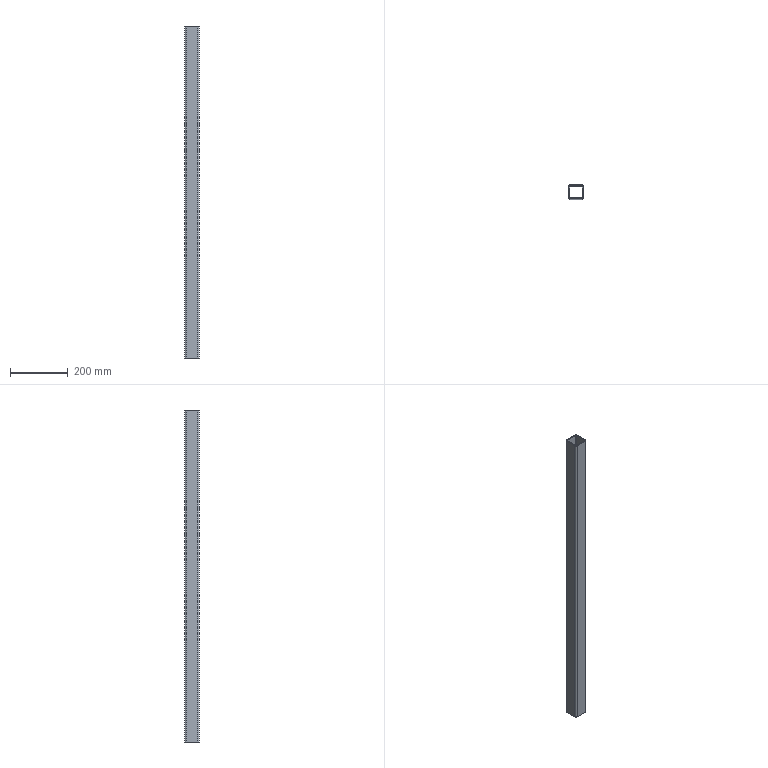Part | STEP file | Square steel 50×50×1150 | 1 solid | 18 faces | box 50 x 50 x 1150 mm | volume 822708 mm3 | plane 10 | cylinder 8 | commonest cylinder face diameters 2 x4 10 x4
STEP:
#1=CARTESIAN_POINT('',(0.,0.,0.));
#2=DIRECTION('',(0.,0.,1.));
#3=DIRECTION('',(1.,0.,0.));
#4=AXIS2_PLACEMENT_3D('',#1,#2,#3);
#5=CARTESIAN_POINT('',(-25.,-20.,575.));
#6=VERTEX_POINT('',#5);
#7=CARTESIAN_POINT('',(-20.,-25.,575.));
#8=VERTEX_POINT('',#7);
#9=CARTESIAN_POINT('',(-20.,-20.,575.));
#10=DIRECTION('',(0.,0.,1.));
#11=DIRECTION('',(1.,0.,0.));
#12=AXIS2_PLACEMENT_3D('',#9,#10,#11);
#13=CIRCLE('',#12,5.);
#14=CARTESIAN_POINT('',(-20.,-20.,575.));
#15=DIRECTION('',(0.,0.,1.));
#16=DIRECTION('',(1.,0.,0.));
#17=AXIS2_PLACEMENT_3D('',#14,#15,#16);
#18=PLANE('',#17);
#19=CARTESIAN_POINT('',(0.,0.));
#20=DIRECTION('',(1.,0.));
#21=AXIS2_PLACEMENT_2D('',#19,#20);
#22=CIRCLE('',#21,5.);
#23=(GEOMETRIC_REPRESENTATION_CONTEXT(2)PARAMETRIC_REPRESENTATION_CONTEXT()REPRESENTATION_CONTEXT('',''));
#24=DEFINITIONAL_REPRESENTATION('',(#22),#23);
#25=PCURVE('',#18,#24);
#26=CARTESIAN_POINT('',(-20.,-20.,575.));
#27=DIRECTION('',(0.,0.,-1.));
#28=DIRECTION('',(-1.,0.,0.));
#29=AXIS2_PLACEMENT_3D('',#26,#27,#28);
#30=CYLINDRICAL_SURFACE('',#29,5.);
#31=CARTESIAN_POINT('',(9.425,0.));
#32=DIRECTION('',(-1.,0.));
#33=VECTOR('',#32,1.);
#34=LINE('',#31,#33);
#35=(GEOMETRIC_REPRESENTATION_CONTEXT(2)PARAMETRIC_REPRESENTATION_CONTEXT()REPRESENTATION_CONTEXT('',''));
#36=DEFINITIONAL_REPRESENTATION('',(#34),#35);
#37=PCURVE('',#30,#36);
#38=SURFACE_CURVE('',#13,(#25,#37),.PCURVE_S1.);
#39=EDGE_CURVE('',#6,#8,#38,.T.);
#40=ORIENTED_EDGE('',*,*,#39,.T.);
#41=CARTESIAN_POINT('',(20.,-25.,575.));
#42=VERTEX_POINT('',#41);
#43=CARTESIAN_POINT('',(-20.,-25.,575.));
#44=DIRECTION('',(1.,0.,0.));
#45=VECTOR('',#44,1.);
#46=LINE('',#43,#45);
#47=CARTESIAN_POINT('',(0.,-5.));
#48=DIRECTION('',(1.,0.));
#49=VECTOR('',#48,1.);
#50=LINE('',#47,#49);
#51=(GEOMETRIC_REPRESENTATION_CONTEXT(2)PARAMETRIC_REPRESENTATION_CONTEXT()REPRESENTATION_CONTEXT('',''));
#52=DEFINITIONAL_REPRESENTATION('',(#50),#51);
#53=PCURVE('',#18,#52);
#54=CARTESIAN_POINT('',(-20.,-25.,575.));
#55=DIRECTION('',(0.,1.,0.));
#56=DIRECTION('',(0.,0.,1.));
#57=AXIS2_PLACEMENT_3D('',#54,#55,#56);
#58=PLANE('',#57);
#59=CARTESIAN_POINT('',(0.,0.));
#60=DIRECTION('',(0.,1.));
#61=VECTOR('',#60,1.);
#62=LINE('',#59,#61);
#63=(GEOMETRIC_REPRESENTATION_CONTEXT(2)PARAMETRIC_REPRESENTATION_CONTEXT()REPRESENTATION_CONTEXT('',''));
#64=DEFINITIONAL_REPRESENTATION('',(#62),#63);
#65=PCURVE('',#58,#64);
#66=SURFACE_CURVE('',#46,(#53,#65),.PCURVE_S1.);
#67=EDGE_CURVE('',#8,#42,#66,.T.);
#68=ORIENTED_EDGE('',*,*,#67,.T.);
#69=CARTESIAN_POINT('',(25.,-20.,575.));
#70=VERTEX_POINT('',#69);
#71=CARTESIAN_POINT('',(20.,-20.,575.));
#72=DIRECTION('',(0.,0.,1.));
#73=DIRECTION('',(-1.,0.,0.));
#74=AXIS2_PLACEMENT_3D('',#71,#72,#73);
#75=CIRCLE('',#74,5.);
#76=CARTESIAN_POINT('',(40.,0.));
#77=DIRECTION('',(-1.,0.));
#78=AXIS2_PLACEMENT_2D('',#76,#77);
#79=CIRCLE('',#78,5.);
#80=(GEOMETRIC_REPRESENTATION_CONTEXT(2)PARAMETRIC_REPRESENTATION_CONTEXT()REPRESENTATION_CONTEXT('',''));
#81=DEFINITIONAL_REPRESENTATION('',(#79),#80);
#82=PCURVE('',#18,#81);
#83=CARTESIAN_POINT('',(20.,-20.,575.));
#84=DIRECTION('',(0.,0.,-1.));
#85=DIRECTION('',(-1.,0.,0.));
#86=AXIS2_PLACEMENT_3D('',#83,#84,#85);
#87=CYLINDRICAL_SURFACE('',#86,5.);
#88=CARTESIAN_POINT('',(6.283,0.));
#89=DIRECTION('',(-1.,0.));
#90=VECTOR('',#89,1.);
#91=LINE('',#88,#90);
#92=(GEOMETRIC_REPRESENTATION_CONTEXT(2)PARAMETRIC_REPRESENTATION_CONTEXT()REPRESENTATION_CONTEXT('',''));
#93=DEFINITIONAL_REPRESENTATION('',(#91),#92);
#94=PCURVE('',#87,#93);
#95=SURFACE_CURVE('',#75,(#82,#94),.PCURVE_S1.);
#96=EDGE_CURVE('',#42,#70,#95,.T.);
#97=ORIENTED_EDGE('',*,*,#96,.T.);
#98=CARTESIAN_POINT('',(25.,20.,575.));
#99=VERTEX_POINT('',#98);
#100=CARTESIAN_POINT('',(25.,20.,575.));
#101=DIRECTION('',(0.,1.,0.));
#102=VECTOR('',#101,1.);
#103=LINE('',#100,#102);
#104=CARTESIAN_POINT('',(45.,40.));
#105=DIRECTION('',(0.,1.));
#106=VECTOR('',#105,1.);
#107=LINE('',#104,#106);
#108=(GEOMETRIC_REPRESENTATION_CONTEXT(2)PARAMETRIC_REPRESENTATION_CONTEXT()REPRESENTATION_CONTEXT('',''));
#109=DEFINITIONAL_REPRESENTATION('',(#107),#108);
#110=PCURVE('',#18,#109);
#111=CARTESIAN_POINT('',(25.,20.,575.));
#112=DIRECTION('',(-1.,0.,0.));
#113=DIRECTION('',(0.,-1.,0.));
#114=AXIS2_PLACEMENT_3D('',#111,#112,#113);
#115=PLANE('',#114);
#116=CARTESIAN_POINT('',(0.,0.));
#117=DIRECTION('',(-1.,0.));
#118=VECTOR('',#117,1.);
#119=LINE('',#116,#118);
#120=(GEOMETRIC_REPRESENTATION_CONTEXT(2)PARAMETRIC_REPRESENTATION_CONTEXT()REPRESENTATION_CONTEXT('',''));
#121=DEFINITIONAL_REPRESENTATION('',(#119),#120);
#122=PCURVE('',#115,#121);
#123=SURFACE_CURVE('',#103,(#110,#122),.PCURVE_S1.);
#124=EDGE_CURVE('',#70,#99,#123,.T.);
#125=ORIENTED_EDGE('',*,*,#124,.T.);
#126=CARTESIAN_POINT('',(20.,25.,575.));
#127=VERTEX_POINT('',#126);
#128=CARTESIAN_POINT('',(20.,20.,575.));
#129=DIRECTION('',(0.,0.,1.));
#130=DIRECTION('',(1.,0.,0.));
#131=AXIS2_PLACEMENT_3D('',#128,#129,#130);
#132=CIRCLE('',#131,5.);
#133=CARTESIAN_POINT('',(40.,40.));
#134=DIRECTION('',(1.,0.));
#135=AXIS2_PLACEMENT_2D('',#133,#134);
#136=CIRCLE('',#135,5.);
#137=(GEOMETRIC_REPRESENTATION_CONTEXT(2)PARAMETRIC_REPRESENTATION_CONTEXT()REPRESENTATION_CONTEXT('',''));
#138=DEFINITIONAL_REPRESENTATION('',(#136),#137);
#139=PCURVE('',#18,#138);
#140=CARTESIAN_POINT('',(20.,20.,575.));
#141=DIRECTION('',(0.,0.,-1.));
#142=DIRECTION('',(-1.,0.,0.));
#143=AXIS2_PLACEMENT_3D('',#140,#141,#142);
#144=CYLINDRICAL_SURFACE('',#143,5.);
#145=CARTESIAN_POINT('',(3.142,0.));
#146=DIRECTION('',(-1.,0.));
#147=VECTOR('',#146,1.);
#148=LINE('',#145,#147);
#149=(GEOMETRIC_REPRESENTATION_CONTEXT(2)PARAMETRIC_REPRESENTATION_CONTEXT()REPRESENTATION_CONTEXT('',''));
#150=DEFINITIONAL_REPRESENTATION('',(#148),#149);
#151=PCURVE('',#144,#150);
#152=SURFACE_CURVE('',#132,(#139,#151),.PCURVE_S1.);
#153=EDGE_CURVE('',#99,#127,#152,.T.);
#154=ORIENTED_EDGE('',*,*,#153,.T.);
#155=CARTESIAN_POINT('',(-20.,25.,575.));
#156=VERTEX_POINT('',#155);
#157=CARTESIAN_POINT('',(-20.,25.,575.));
#158=DIRECTION('',(-1.,0.,0.));
#159=VECTOR('',#158,1.);
#160=LINE('',#157,#159);
#161=CARTESIAN_POINT('',(0.,45.));
#162=DIRECTION('',(-1.,0.));
#163=VECTOR('',#162,1.);
#164=LINE('',#161,#163);
#165=(GEOMETRIC_REPRESENTATION_CONTEXT(2)PARAMETRIC_REPRESENTATION_CONTEXT()REPRESENTATION_CONTEXT('',''));
#166=DEFINITIONAL_REPRESENTATION('',(#164),#165);
#167=PCURVE('',#18,#166);
#168=CARTESIAN_POINT('',(-20.,25.,575.));
#169=DIRECTION('',(0.,-1.,0.));
#170=DIRECTION('',(0.,0.,-1.));
#171=AXIS2_PLACEMENT_3D('',#168,#169,#170);
#172=PLANE('',#171);
#173=CARTESIAN_POINT('',(0.,0.));
#174=DIRECTION('',(0.,-1.));
#175=VECTOR('',#174,1.);
#176=LINE('',#173,#175);
#177=(GEOMETRIC_REPRESENTATION_CONTEXT(2)PARAMETRIC_REPRESENTATION_CONTEXT()REPRESENTATION_CONTEXT('',''));
#178=DEFINITIONAL_REPRESENTATION('',(#176),#177);
#179=PCURVE('',#172,#178);
#180=SURFACE_CURVE('',#160,(#167,#179),.PCURVE_S1.);
#181=EDGE_CURVE('',#127,#156,#180,.T.);
#182=ORIENTED_EDGE('',*,*,#181,.T.);
#183=CARTESIAN_POINT('',(-25.,20.,575.));
#184=VERTEX_POINT('',#183);
#185=CARTESIAN_POINT('',(-20.,20.,575.));
#186=DIRECTION('',(0.,0.,1.));
#187=DIRECTION('',(-1.,0.,0.));
#188=AXIS2_PLACEMENT_3D('',#185,#186,#187);
#189=CIRCLE('',#188,5.);
#190=CARTESIAN_POINT('',(0.,40.));
#191=DIRECTION('',(-1.,0.));
#192=AXIS2_PLACEMENT_2D('',#190,#191);
#193=CIRCLE('',#192,5.);
#194=(GEOMETRIC_REPRESENTATION_CONTEXT(2)PARAMETRIC_REPRESENTATION_CONTEXT()REPRESENTATION_CONTEXT('',''));
#195=DEFINITIONAL_REPRESENTATION('',(#193),#194);
#196=PCURVE('',#18,#195);
#197=CARTESIAN_POINT('',(-20.,20.,575.));
#198=DIRECTION('',(0.,0.,-1.));
#199=DIRECTION('',(-1.,0.,0.));
#200=AXIS2_PLACEMENT_3D('',#197,#198,#199);
#201=CYLINDRICAL_SURFACE('',#200,5.);
#202=CARTESIAN_POINT('',(6.283,0.));
#203=DIRECTION('',(-1.,0.));
#204=VECTOR('',#203,1.);
#205=LINE('',#202,#204);
#206=(GEOMETRIC_REPRESENTATION_CONTEXT(2)PARAMETRIC_REPRESENTATION_CONTEXT()REPRESENTATION_CONTEXT('',''));
#207=DEFINITIONAL_REPRESENTATION('',(#205),#206);
#208=PCURVE('',#201,#207);
#209=SURFACE_CURVE('',#189,(#196,#208),.PCURVE_S1.);
#210=EDGE_CURVE('',#156,#184,#209,.T.);
#211=ORIENTED_EDGE('',*,*,#210,.T.);
#212=CARTESIAN_POINT('',(-25.,20.,575.));
#213=DIRECTION('',(0.,-1.,0.));
#214=VECTOR('',#213,1.);
#215=LINE('',#212,#214);
#216=CARTESIAN_POINT('',(-5.,40.));
#217=DIRECTION('',(0.,-1.));
#218=VECTOR('',#217,1.);
#219=LINE('',#216,#218);
#220=(GEOMETRIC_REPRESENTATION_CONTEXT(2)PARAMETRIC_REPRESENTATION_CONTEXT()REPRESENTATION_CONTEXT('',''));
#221=DEFINITIONAL_REPRESENTATION('',(#219),#220);
#222=PCURVE('',#18,#221);
#223=CARTESIAN_POINT('',(-25.,20.,575.));
#224=DIRECTION('',(1.,0.,0.));
#225=DIRECTION('',(0.,1.,0.));
#226=AXIS2_PLACEMENT_3D('',#223,#224,#225);
#227=PLANE('',#226);
#228=CARTESIAN_POINT('',(0.,0.));
#229=DIRECTION('',(-1.,0.));
#230=VECTOR('',#229,1.);
#231=LINE('',#228,#230);
#232=(GEOMETRIC_REPRESENTATION_CONTEXT(2)PARAMETRIC_REPRESENTATION_CONTEXT()REPRESENTATION_CONTEXT('',''));
#233=DEFINITIONAL_REPRESENTATION('',(#231),#232);
#234=PCURVE('',#227,#233);
#235=SURFACE_CURVE('',#215,(#222,#234),.PCURVE_S1.);
#236=EDGE_CURVE('',#184,#6,#235,.T.);
#237=ORIENTED_EDGE('',*,*,#236,.T.);
#238=EDGE_LOOP('',(#40,#68,#97,#125,#154,#182,#211,#237));
#239=FACE_BOUND('',#238,.T.);
#240=CARTESIAN_POINT('',(-21.,20.,575.));
#241=VERTEX_POINT('',#240);
#242=CARTESIAN_POINT('',(-21.,-20.,575.));
#243=VERTEX_POINT('',#242);
#244=CARTESIAN_POINT('',(-21.,20.,575.));
#245=DIRECTION('',(0.,-1.,0.));
#246=VECTOR('',#245,1.);
#247=LINE('',#244,#246);
#248=CARTESIAN_POINT('',(-1.,40.));
#249=DIRECTION('',(0.,-1.));
#250=VECTOR('',#249,1.);
#251=LINE('',#248,#250);
#252=(GEOMETRIC_REPRESENTATION_CONTEXT(2)PARAMETRIC_REPRESENTATION_CONTEXT()REPRESENTATION_CONTEXT('',''));
#253=DEFINITIONAL_REPRESENTATION('',(#251),#252);
#254=PCURVE('',#18,#253);
#255=CARTESIAN_POINT('',(-21.,20.,575.));
#256=DIRECTION('',(1.,0.,0.));
#257=DIRECTION('',(0.,1.,0.));
#258=AXIS2_PLACEMENT_3D('',#255,#256,#257);
#259=PLANE('',#258);
#260=CARTESIAN_POINT('',(0.,0.));
#261=DIRECTION('',(-1.,0.));
#262=VECTOR('',#261,1.);
#263=LINE('',#260,#262);
#264=(GEOMETRIC_REPRESENTATION_CONTEXT(2)PARAMETRIC_REPRESENTATION_CONTEXT()REPRESENTATION_CONTEXT('',''));
#265=DEFINITIONAL_REPRESENTATION('',(#263),#264);
#266=PCURVE('',#259,#265);
#267=SURFACE_CURVE('',#247,(#254,#266),.PCURVE_S1.);
#268=EDGE_CURVE('',#241,#243,#267,.T.);
#269=ORIENTED_EDGE('',*,*,#268,.F.);
#270=CARTESIAN_POINT('',(-20.,21.,575.));
#271=VERTEX_POINT('',#270);
#272=CARTESIAN_POINT('',(-20.,20.,575.));
#273=DIRECTION('',(0.,0.,1.));
#274=DIRECTION('',(-1.,0.,0.));
#275=AXIS2_PLACEMENT_3D('',#272,#273,#274);
#276=CIRCLE('',#275,1.);
#277=CARTESIAN_POINT('',(0.,40.));
#278=DIRECTION('',(-1.,0.));
#279=AXIS2_PLACEMENT_2D('',#277,#278);
#280=CIRCLE('',#279,1.);
#281=(GEOMETRIC_REPRESENTATION_CONTEXT(2)PARAMETRIC_REPRESENTATION_CONTEXT()REPRESENTATION_CONTEXT('',''));
#282=DEFINITIONAL_REPRESENTATION('',(#280),#281);
#283=PCURVE('',#18,#282);
#284=CARTESIAN_POINT('',(-20.,20.,575.));
#285=DIRECTION('',(0.,0.,-1.));
#286=DIRECTION('',(-1.,0.,0.));
#287=AXIS2_PLACEMENT_3D('',#284,#285,#286);
#288=CYLINDRICAL_SURFACE('',#287,1.);
#289=CARTESIAN_POINT('',(6.283,0.));
#290=DIRECTION('',(-1.,0.));
#291=VECTOR('',#290,1.);
#292=LINE('',#289,#291);
#293=(GEOMETRIC_REPRESENTATION_CONTEXT(2)PARAMETRIC_REPRESENTATION_CONTEXT()REPRESENTATION_CONTEXT('',''));
#294=DEFINITIONAL_REPRESENTATION('',(#292),#293);
#295=PCURVE('',#288,#294);
#296=SURFACE_CURVE('',#276,(#283,#295),.PCURVE_S1.);
#297=EDGE_CURVE('',#271,#241,#296,.T.);
#298=ORIENTED_EDGE('',*,*,#297,.F.);
#299=CARTESIAN_POINT('',(20.,21.,575.));
#300=VERTEX_POINT('',#299);
#301=CARTESIAN_POINT('',(-20.,21.,575.));
#302=DIRECTION('',(-1.,0.,0.));
#303=VECTOR('',#302,1.);
#304=LINE('',#301,#303);
#305=CARTESIAN_POINT('',(0.,41.));
#306=DIRECTION('',(-1.,0.));
#307=VECTOR('',#306,1.);
#308=LINE('',#305,#307);
#309=(GEOMETRIC_REPRESENTATION_CONTEXT(2)PARAMETRIC_REPRESENTATION_CONTEXT()REPRESENTATION_CONTEXT('',''));
#310=DEFINITIONAL_REPRESENTATION('',(#308),#309);
#311=PCURVE('',#18,#310);
#312=CARTESIAN_POINT('',(-20.,21.,575.));
#313=DIRECTION('',(0.,-1.,0.));
#314=DIRECTION('',(0.,0.,-1.));
#315=AXIS2_PLACEMENT_3D('',#312,#313,#314);
#316=PLANE('',#315);
#317=CARTESIAN_POINT('',(0.,0.));
#318=DIRECTION('',(0.,-1.));
#319=VECTOR('',#318,1.);
#320=LINE('',#317,#319);
#321=(GEOMETRIC_REPRESENTATION_CONTEXT(2)PARAMETRIC_REPRESENTATION_CONTEXT()REPRESENTATION_CONTEXT('',''));
#322=DEFINITIONAL_REPRESENTATION('',(#320),#321);
#323=PCURVE('',#316,#322);
#324=SURFACE_CURVE('',#304,(#311,#323),.PCURVE_S1.);
#325=EDGE_CURVE('',#300,#271,#324,.T.);
#326=ORIENTED_EDGE('',*,*,#325,.F.);
#327=CARTESIAN_POINT('',(21.,20.,575.));
#328=VERTEX_POINT('',#327);
#329=CARTESIAN_POINT('',(20.,20.,575.));
#330=DIRECTION('',(0.,0.,1.));
#331=DIRECTION('',(1.,0.,0.));
#332=AXIS2_PLACEMENT_3D('',#329,#330,#331);
#333=CIRCLE('',#332,1.);
#334=CARTESIAN_POINT('',(40.,40.));
#335=DIRECTION('',(1.,0.));
#336=AXIS2_PLACEMENT_2D('',#334,#335);
#337=CIRCLE('',#336,1.);
#338=(GEOMETRIC_REPRESENTATION_CONTEXT(2)PARAMETRIC_REPRESENTATION_CONTEXT()REPRESENTATION_CONTEXT('',''));
#339=DEFINITIONAL_REPRESENTATION('',(#337),#338);
#340=PCURVE('',#18,#339);
#341=CARTESIAN_POINT('',(20.,20.,575.));
#342=DIRECTION('',(0.,0.,-1.));
#343=DIRECTION('',(-1.,0.,0.));
#344=AXIS2_PLACEMENT_3D('',#341,#342,#343);
#345=CYLINDRICAL_SURFACE('',#344,1.);
#346=CARTESIAN_POINT('',(3.142,0.));
#347=DIRECTION('',(-1.,0.));
#348=VECTOR('',#347,1.);
#349=LINE('',#346,#348);
#350=(GEOMETRIC_REPRESENTATION_CONTEXT(2)PARAMETRIC_REPRESENTATION_CONTEXT()REPRESENTATION_CONTEXT('',''));
#351=DEFINITIONAL_REPRESENTATION('',(#349),#350);
#352=PCURVE('',#345,#351);
#353=SURFACE_CURVE('',#333,(#340,#352),.PCURVE_S1.);
#354=EDGE_CURVE('',#328,#300,#353,.T.);
#355=ORIENTED_EDGE('',*,*,#354,.F.);
#356=CARTESIAN_POINT('',(21.,-20.,575.));
#357=VERTEX_POINT('',#356);
#358=CARTESIAN_POINT('',(21.,20.,575.));
#359=DIRECTION('',(0.,1.,0.));
#360=VECTOR('',#359,1.);
#361=LINE('',#358,#360);
#362=CARTESIAN_POINT('',(41.,40.));
#363=DIRECTION('',(0.,1.));
#364=VECTOR('',#363,1.);
#365=LINE('',#362,#364);
#366=(GEOMETRIC_REPRESENTATION_CONTEXT(2)PARAMETRIC_REPRESENTATION_CONTEXT()REPRESENTATION_CONTEXT('',''));
#367=DEFINITIONAL_REPRESENTATION('',(#365),#366);
#368=PCURVE('',#18,#367);
#369=CARTESIAN_POINT('',(21.,20.,575.));
#370=DIRECTION('',(-1.,0.,0.));
#371=DIRECTION('',(0.,0.,1.));
#372=AXIS2_PLACEMENT_3D('',#369,#370,#371);
#373=PLANE('',#372);
#374=CARTESIAN_POINT('',(0.,0.));
#375=DIRECTION('',(0.,1.));
#376=VECTOR('',#375,1.);
#377=LINE('',#374,#376);
#378=(GEOMETRIC_REPRESENTATION_CONTEXT(2)PARAMETRIC_REPRESENTATION_CONTEXT()REPRESENTATION_CONTEXT('',''));
#379=DEFINITIONAL_REPRESENTATION('',(#377),#378);
#380=PCURVE('',#373,#379);
#381=SURFACE_CURVE('',#361,(#368,#380),.PCURVE_S1.);
#382=EDGE_CURVE('',#357,#328,#381,.T.);
#383=ORIENTED_EDGE('',*,*,#382,.F.);
#384=CARTESIAN_POINT('',(20.,-21.,575.));
#385=VERTEX_POINT('',#384);
#386=CARTESIAN_POINT('',(20.,-20.,575.));
#387=DIRECTION('',(0.,0.,1.));
#388=DIRECTION('',(-1.,0.,0.));
#389=AXIS2_PLACEMENT_3D('',#386,#387,#388);
#390=CIRCLE('',#389,1.);
#391=CARTESIAN_POINT('',(40.,0.));
#392=DIRECTION('',(-1.,0.));
#393=AXIS2_PLACEMENT_2D('',#391,#392);
#394=CIRCLE('',#393,1.);
#395=(GEOMETRIC_REPRESENTATION_CONTEXT(2)PARAMETRIC_REPRESENTATION_CONTEXT()REPRESENTATION_CONTEXT('',''));
#396=DEFINITIONAL_REPRESENTATION('',(#394),#395);
#397=PCURVE('',#18,#396);
#398=CARTESIAN_POINT('',(20.,-20.,575.));
#399=DIRECTION('',(0.,0.,-1.));
#400=DIRECTION('',(-1.,0.,0.));
#401=AXIS2_PLACEMENT_3D('',#398,#399,#400);
#402=CYLINDRICAL_SURFACE('',#401,1.);
#403=CARTESIAN_POINT('',(6.283,0.));
#404=DIRECTION('',(-1.,0.));
#405=VECTOR('',#404,1.);
#406=LINE('',#403,#405);
#407=(GEOMETRIC_REPRESENTATION_CONTEXT(2)PARAMETRIC_REPRESENTATION_CONTEXT()REPRESENTATION_CONTEXT('',''));
#408=DEFINITIONAL_REPRESENTATION('',(#406),#407);
#409=PCURVE('',#402,#408);
#410=SURFACE_CURVE('',#390,(#397,#409),.PCURVE_S1.);
#411=EDGE_CURVE('',#385,#357,#410,.T.);
#412=ORIENTED_EDGE('',*,*,#411,.F.);
#413=CARTESIAN_POINT('',(-20.,-21.,575.));
#414=VERTEX_POINT('',#413);
#415=CARTESIAN_POINT('',(-20.,-21.,575.));
#416=DIRECTION('',(1.,0.,0.));
#417=VECTOR('',#416,1.);
#418=LINE('',#415,#417);
#419=CARTESIAN_POINT('',(0.,-1.));
#420=DIRECTION('',(1.,0.));
#421=VECTOR('',#420,1.);
#422=LINE('',#419,#421);
#423=(GEOMETRIC_REPRESENTATION_CONTEXT(2)PARAMETRIC_REPRESENTATION_CONTEXT()REPRESENTATION_CONTEXT('',''));
#424=DEFINITIONAL_REPRESENTATION('',(#422),#423);
#425=PCURVE('',#18,#424);
#426=CARTESIAN_POINT('',(-20.,-21.,575.));
#427=DIRECTION('',(0.,1.,0.));
#428=DIRECTION('',(0.,0.,1.));
#429=AXIS2_PLACEMENT_3D('',#426,#427,#428);
#430=PLANE('',#429);
#431=CARTESIAN_POINT('',(0.,0.));
#432=DIRECTION('',(0.,1.));
#433=VECTOR('',#432,1.);
#434=LINE('',#431,#433);
#435=(GEOMETRIC_REPRESENTATION_CONTEXT(2)PARAMETRIC_REPRESENTATION_CONTEXT()REPRESENTATION_CONTEXT('',''));
#436=DEFINITIONAL_REPRESENTATION('',(#434),#435);
#437=PCURVE('',#430,#436);
#438=SURFACE_CURVE('',#418,(#425,#437),.PCURVE_S1.);
#439=EDGE_CURVE('',#414,#385,#438,.T.);
#440=ORIENTED_EDGE('',*,*,#439,.F.);
#441=CARTESIAN_POINT('',(-20.,-20.,575.));
#442=DIRECTION('',(0.,0.,1.));
#443=DIRECTION('',(1.,0.,0.));
#444=AXIS2_PLACEMENT_3D('',#441,#442,#443);
#445=CIRCLE('',#444,1.);
#446=CARTESIAN_POINT('',(0.,0.));
#447=DIRECTION('',(1.,0.));
#448=AXIS2_PLACEMENT_2D('',#446,#447);
#449=CIRCLE('',#448,1.);
#450=(GEOMETRIC_REPRESENTATION_CONTEXT(2)PARAMETRIC_REPRESENTATION_CONTEXT()REPRESENTATION_CONTEXT('',''));
#451=DEFINITIONAL_REPRESENTATION('',(#449),#450);
#452=PCURVE('',#18,#451);
#453=CARTESIAN_POINT('',(-20.,-20.,575.));
#454=DIRECTION('',(0.,0.,-1.));
#455=DIRECTION('',(-1.,0.,0.));
#456=AXIS2_PLACEMENT_3D('',#453,#454,#455);
#457=CYLINDRICAL_SURFACE('',#456,1.);
#458=CARTESIAN_POINT('',(9.425,0.));
#459=DIRECTION('',(-1.,0.));
#460=VECTOR('',#459,1.);
#461=LINE('',#458,#460);
#462=(GEOMETRIC_REPRESENTATION_CONTEXT(2)PARAMETRIC_REPRESENTATION_CONTEXT()REPRESENTATION_CONTEXT('',''));
#463=DEFINITIONAL_REPRESENTATION('',(#461),#462);
#464=PCURVE('',#457,#463);
#465=SURFACE_CURVE('',#445,(#452,#464),.PCURVE_S1.);
#466=EDGE_CURVE('',#243,#414,#465,.T.);
#467=ORIENTED_EDGE('',*,*,#466,.F.);
#468=EDGE_LOOP('',(#269,#298,#326,#355,#383,#412,#440,#467));
#469=FACE_BOUND('',#468,.T.);
#470=ADVANCED_FACE('',(#239,#469),#18,.T.);
#471=CARTESIAN_POINT('',(-25.,-20.,-575.));
#472=VERTEX_POINT('',#471);
#473=CARTESIAN_POINT('',(-20.,-25.,-575.));
#474=VERTEX_POINT('',#473);
#475=CARTESIAN_POINT('',(-20.,-20.,-575.));
#476=DIRECTION('',(0.,0.,1.));
#477=DIRECTION('',(1.,0.,0.));
#478=AXIS2_PLACEMENT_3D('',#475,#476,#477);
#479=CIRCLE('',#478,5.);
#480=CARTESIAN_POINT('',(-20.,-20.,-575.));
#481=DIRECTION('',(0.,0.,1.));
#482=DIRECTION('',(1.,0.,0.));
#483=AXIS2_PLACEMENT_3D('',#480,#481,#482);
#484=PLANE('',#483);
#485=CARTESIAN_POINT('',(0.,0.));
#486=DIRECTION('',(1.,0.));
#487=AXIS2_PLACEMENT_2D('',#485,#486);
#488=CIRCLE('',#487,5.);
#489=(GEOMETRIC_REPRESENTATION_CONTEXT(2)PARAMETRIC_REPRESENTATION_CONTEXT()REPRESENTATION_CONTEXT('',''));
#490=DEFINITIONAL_REPRESENTATION('',(#488),#489);
#491=PCURVE('',#484,#490);
#492=CARTESIAN_POINT('',(9.425,1150.));
#493=DIRECTION('',(-1.,0.));
#494=VECTOR('',#493,1.);
#495=LINE('',#492,#494);
#496=(GEOMETRIC_REPRESENTATION_CONTEXT(2)PARAMETRIC_REPRESENTATION_CONTEXT()REPRESENTATION_CONTEXT('',''));
#497=DEFINITIONAL_REPRESENTATION('',(#495),#496);
#498=PCURVE('',#30,#497);
#499=SURFACE_CURVE('',#479,(#491,#498),.PCURVE_S1.);
#500=EDGE_CURVE('',#472,#474,#499,.T.);
#501=ORIENTED_EDGE('',*,*,#500,.F.);
#502=CARTESIAN_POINT('',(-25.,20.,-575.));
#503=VERTEX_POINT('',#502);
#504=CARTESIAN_POINT('',(-25.,20.,-575.));
#505=DIRECTION('',(0.,-1.,0.));
#506=VECTOR('',#505,1.);
#507=LINE('',#504,#506);
#508=CARTESIAN_POINT('',(-5.,40.));
#509=DIRECTION('',(0.,-1.));
#510=VECTOR('',#509,1.);
#511=LINE('',#508,#510);
#512=(GEOMETRIC_REPRESENTATION_CONTEXT(2)PARAMETRIC_REPRESENTATION_CONTEXT()REPRESENTATION_CONTEXT('',''));
#513=DEFINITIONAL_REPRESENTATION('',(#511),#512);
#514=PCURVE('',#484,#513);
#515=CARTESIAN_POINT('',(0.,-1150.));
#516=DIRECTION('',(-1.,0.));
#517=VECTOR('',#516,1.);
#518=LINE('',#515,#517);
#519=(GEOMETRIC_REPRESENTATION_CONTEXT(2)PARAMETRIC_REPRESENTATION_CONTEXT()REPRESENTATION_CONTEXT('',''));
#520=DEFINITIONAL_REPRESENTATION('',(#518),#519);
#521=PCURVE('',#227,#520);
#522=SURFACE_CURVE('',#507,(#514,#521),.PCURVE_S1.);
#523=EDGE_CURVE('',#503,#472,#522,.T.);
#524=ORIENTED_EDGE('',*,*,#523,.F.);
#525=CARTESIAN_POINT('',(-20.,25.,-575.));
#526=VERTEX_POINT('',#525);
#527=CARTESIAN_POINT('',(-20.,20.,-575.));
#528=DIRECTION('',(0.,0.,1.));
#529=DIRECTION('',(-1.,0.,0.));
#530=AXIS2_PLACEMENT_3D('',#527,#528,#529);
#531=CIRCLE('',#530,5.);
#532=CARTESIAN_POINT('',(0.,40.));
#533=DIRECTION('',(-1.,0.));
#534=AXIS2_PLACEMENT_2D('',#532,#533);
#535=CIRCLE('',#534,5.);
#536=(GEOMETRIC_REPRESENTATION_CONTEXT(2)PARAMETRIC_REPRESENTATION_CONTEXT()REPRESENTATION_CONTEXT('',''));
#537=DEFINITIONAL_REPRESENTATION('',(#535),#536);
#538=PCURVE('',#484,#537);
#539=CARTESIAN_POINT('',(6.283,1150.));
#540=DIRECTION('',(-1.,0.));
#541=VECTOR('',#540,1.);
#542=LINE('',#539,#541);
#543=(GEOMETRIC_REPRESENTATION_CONTEXT(2)PARAMETRIC_REPRESENTATION_CONTEXT()REPRESENTATION_CONTEXT('',''));
#544=DEFINITIONAL_REPRESENTATION('',(#542),#543);
#545=PCURVE('',#201,#544);
#546=SURFACE_CURVE('',#531,(#538,#545),.PCURVE_S1.);
#547=EDGE_CURVE('',#526,#503,#546,.T.);
#548=ORIENTED_EDGE('',*,*,#547,.F.);
#549=CARTESIAN_POINT('',(20.,25.,-575.));
#550=VERTEX_POINT('',#549);
#551=CARTESIAN_POINT('',(-20.,25.,-575.));
#552=DIRECTION('',(-1.,0.,0.));
#553=VECTOR('',#552,1.);
#554=LINE('',#551,#553);
#555=CARTESIAN_POINT('',(0.,45.));
#556=DIRECTION('',(-1.,0.));
#557=VECTOR('',#556,1.);
#558=LINE('',#555,#557);
#559=(GEOMETRIC_REPRESENTATION_CONTEXT(2)PARAMETRIC_REPRESENTATION_CONTEXT()REPRESENTATION_CONTEXT('',''));
#560=DEFINITIONAL_REPRESENTATION('',(#558),#559);
#561=PCURVE('',#484,#560);
#562=CARTESIAN_POINT('',(1150.,0.));
#563=DIRECTION('',(0.,-1.));
#564=VECTOR('',#563,1.);
#565=LINE('',#562,#564);
#566=(GEOMETRIC_REPRESENTATION_CONTEXT(2)PARAMETRIC_REPRESENTATION_CONTEXT()REPRESENTATION_CONTEXT('',''));
#567=DEFINITIONAL_REPRESENTATION('',(#565),#566);
#568=PCURVE('',#172,#567);
#569=SURFACE_CURVE('',#554,(#561,#568),.PCURVE_S1.);
#570=EDGE_CURVE('',#550,#526,#569,.T.);
#571=ORIENTED_EDGE('',*,*,#570,.F.);
#572=CARTESIAN_POINT('',(25.,20.,-575.));
#573=VERTEX_POINT('',#572);
#574=CARTESIAN_POINT('',(20.,20.,-575.));
#575=DIRECTION('',(0.,0.,1.));
#576=DIRECTION('',(1.,0.,0.));
#577=AXIS2_PLACEMENT_3D('',#574,#575,#576);
#578=CIRCLE('',#577,5.);
#579=CARTESIAN_POINT('',(40.,40.));
#580=DIRECTION('',(1.,0.));
#581=AXIS2_PLACEMENT_2D('',#579,#580);
#582=CIRCLE('',#581,5.);
#583=(GEOMETRIC_REPRESENTATION_CONTEXT(2)PARAMETRIC_REPRESENTATION_CONTEXT()REPRESENTATION_CONTEXT('',''));
#584=DEFINITIONAL_REPRESENTATION('',(#582),#583);
#585=PCURVE('',#484,#584);
#586=CARTESIAN_POINT('',(3.142,1150.));
#587=DIRECTION('',(-1.,0.));
#588=VECTOR('',#587,1.);
#589=LINE('',#586,#588);
#590=(GEOMETRIC_REPRESENTATION_CONTEXT(2)PARAMETRIC_REPRESENTATION_CONTEXT()REPRESENTATION_CONTEXT('',''));
#591=DEFINITIONAL_REPRESENTATION('',(#589),#590);
#592=PCURVE('',#144,#591);
#593=SURFACE_CURVE('',#578,(#585,#592),.PCURVE_S1.);
#594=EDGE_CURVE('',#573,#550,#593,.T.);
#595=ORIENTED_EDGE('',*,*,#594,.F.);
#596=CARTESIAN_POINT('',(25.,-20.,-575.));
#597=VERTEX_POINT('',#596);
#598=CARTESIAN_POINT('',(25.,20.,-575.));
#599=DIRECTION('',(0.,1.,0.));
#600=VECTOR('',#599,1.);
#601=LINE('',#598,#600);
#602=CARTESIAN_POINT('',(45.,40.));
#603=DIRECTION('',(0.,1.));
#604=VECTOR('',#603,1.);
#605=LINE('',#602,#604);
#606=(GEOMETRIC_REPRESENTATION_CONTEXT(2)PARAMETRIC_REPRESENTATION_CONTEXT()REPRESENTATION_CONTEXT('',''));
#607=DEFINITIONAL_REPRESENTATION('',(#605),#606);
#608=PCURVE('',#484,#607);
#609=CARTESIAN_POINT('',(0.,-1150.));
#610=DIRECTION('',(-1.,0.));
#611=VECTOR('',#610,1.);
#612=LINE('',#609,#611);
#613=(GEOMETRIC_REPRESENTATION_CONTEXT(2)PARAMETRIC_REPRESENTATION_CONTEXT()REPRESENTATION_CONTEXT('',''));
#614=DEFINITIONAL_REPRESENTATION('',(#612),#613);
#615=PCURVE('',#115,#614);
#616=SURFACE_CURVE('',#601,(#608,#615),.PCURVE_S1.);
#617=EDGE_CURVE('',#597,#573,#616,.T.);
#618=ORIENTED_EDGE('',*,*,#617,.F.);
#619=CARTESIAN_POINT('',(20.,-25.,-575.));
#620=VERTEX_POINT('',#619);
#621=CARTESIAN_POINT('',(20.,-20.,-575.));
#622=DIRECTION('',(0.,0.,1.));
#623=DIRECTION('',(-1.,0.,0.));
#624=AXIS2_PLACEMENT_3D('',#621,#622,#623);
#625=CIRCLE('',#624,5.);
#626=CARTESIAN_POINT('',(40.,0.));
#627=DIRECTION('',(-1.,0.));
#628=AXIS2_PLACEMENT_2D('',#626,#627);
#629=CIRCLE('',#628,5.);
#630=(GEOMETRIC_REPRESENTATION_CONTEXT(2)PARAMETRIC_REPRESENTATION_CONTEXT()REPRESENTATION_CONTEXT('',''));
#631=DEFINITIONAL_REPRESENTATION('',(#629),#630);
#632=PCURVE('',#484,#631);
#633=CARTESIAN_POINT('',(6.283,1150.));
#634=DIRECTION('',(-1.,0.));
#635=VECTOR('',#634,1.);
#636=LINE('',#633,#635);
#637=(GEOMETRIC_REPRESENTATION_CONTEXT(2)PARAMETRIC_REPRESENTATION_CONTEXT()REPRESENTATION_CONTEXT('',''));
#638=DEFINITIONAL_REPRESENTATION('',(#636),#637);
#639=PCURVE('',#87,#638);
#640=SURFACE_CURVE('',#625,(#632,#639),.PCURVE_S1.);
#641=EDGE_CURVE('',#620,#597,#640,.T.);
#642=ORIENTED_EDGE('',*,*,#641,.F.);
#643=CARTESIAN_POINT('',(-20.,-25.,-575.));
#644=DIRECTION('',(1.,0.,0.));
#645=VECTOR('',#644,1.);
#646=LINE('',#643,#645);
#647=CARTESIAN_POINT('',(0.,-5.));
#648=DIRECTION('',(1.,0.));
#649=VECTOR('',#648,1.);
#650=LINE('',#647,#649);
#651=(GEOMETRIC_REPRESENTATION_CONTEXT(2)PARAMETRIC_REPRESENTATION_CONTEXT()REPRESENTATION_CONTEXT('',''));
#652=DEFINITIONAL_REPRESENTATION('',(#650),#651);
#653=PCURVE('',#484,#652);
#654=CARTESIAN_POINT('',(-1150.,0.));
#655=DIRECTION('',(0.,1.));
#656=VECTOR('',#655,1.);
#657=LINE('',#654,#656);
#658=(GEOMETRIC_REPRESENTATION_CONTEXT(2)PARAMETRIC_REPRESENTATION_CONTEXT()REPRESENTATION_CONTEXT('',''));
#659=DEFINITIONAL_REPRESENTATION('',(#657),#658);
#660=PCURVE('',#58,#659);
#661=SURFACE_CURVE('',#646,(#653,#660),.PCURVE_S1.);
#662=EDGE_CURVE('',#474,#620,#661,.T.);
#663=ORIENTED_EDGE('',*,*,#662,.F.);
#664=EDGE_LOOP('',(#501,#524,#548,#571,#595,#618,#642,#663));
#665=FACE_BOUND('',#664,.T.);
#666=CARTESIAN_POINT('',(-20.,21.,-575.));
#667=VERTEX_POINT('',#666);
#668=CARTESIAN_POINT('',(-21.,20.,-575.));
#669=VERTEX_POINT('',#668);
#670=CARTESIAN_POINT('',(-20.,20.,-575.));
#671=DIRECTION('',(0.,0.,1.));
#672=DIRECTION('',(-1.,0.,0.));
#673=AXIS2_PLACEMENT_3D('',#670,#671,#672);
#674=CIRCLE('',#673,1.);
#675=CARTESIAN_POINT('',(0.,40.));
#676=DIRECTION('',(-1.,0.));
#677=AXIS2_PLACEMENT_2D('',#675,#676);
#678=CIRCLE('',#677,1.);
#679=(GEOMETRIC_REPRESENTATION_CONTEXT(2)PARAMETRIC_REPRESENTATION_CONTEXT()REPRESENTATION_CONTEXT('',''));
#680=DEFINITIONAL_REPRESENTATION('',(#678),#679);
#681=PCURVE('',#484,#680);
#682=CARTESIAN_POINT('',(6.283,1150.));
#683=DIRECTION('',(-1.,0.));
#684=VECTOR('',#683,1.);
#685=LINE('',#682,#684);
#686=(GEOMETRIC_REPRESENTATION_CONTEXT(2)PARAMETRIC_REPRESENTATION_CONTEXT()REPRESENTATION_CONTEXT('',''));
#687=DEFINITIONAL_REPRESENTATION('',(#685),#686);
#688=PCURVE('',#288,#687);
#689=SURFACE_CURVE('',#674,(#681,#688),.PCURVE_S1.);
#690=EDGE_CURVE('',#667,#669,#689,.T.);
#691=ORIENTED_EDGE('',*,*,#690,.T.);
#692=CARTESIAN_POINT('',(-21.,-20.,-575.));
#693=VERTEX_POINT('',#692);
#694=CARTESIAN_POINT('',(-21.,20.,-575.));
#695=DIRECTION('',(0.,-1.,0.));
#696=VECTOR('',#695,1.);
#697=LINE('',#694,#696);
#698=CARTESIAN_POINT('',(-1.,40.));
#699=DIRECTION('',(0.,-1.));
#700=VECTOR('',#699,1.);
#701=LINE('',#698,#700);
#702=(GEOMETRIC_REPRESENTATION_CONTEXT(2)PARAMETRIC_REPRESENTATION_CONTEXT()REPRESENTATION_CONTEXT('',''));
#703=DEFINITIONAL_REPRESENTATION('',(#701),#702);
#704=PCURVE('',#484,#703);
#705=CARTESIAN_POINT('',(0.,-1150.));
#706=DIRECTION('',(-1.,0.));
#707=VECTOR('',#706,1.);
#708=LINE('',#705,#707);
#709=(GEOMETRIC_REPRESENTATION_CONTEXT(2)PARAMETRIC_REPRESENTATION_CONTEXT()REPRESENTATION_CONTEXT('',''));
#710=DEFINITIONAL_REPRESENTATION('',(#708),#709);
#711=PCURVE('',#259,#710);
#712=SURFACE_CURVE('',#697,(#704,#711),.PCURVE_S1.);
#713=EDGE_CURVE('',#669,#693,#712,.T.);
#714=ORIENTED_EDGE('',*,*,#713,.T.);
#715=CARTESIAN_POINT('',(-20.,-21.,-575.));
#716=VERTEX_POINT('',#715);
#717=CARTESIAN_POINT('',(-20.,-20.,-575.));
#718=DIRECTION('',(0.,0.,1.));
#719=DIRECTION('',(1.,0.,0.));
#720=AXIS2_PLACEMENT_3D('',#717,#718,#719);
#721=CIRCLE('',#720,1.);
#722=CARTESIAN_POINT('',(0.,0.));
#723=DIRECTION('',(1.,0.));
#724=AXIS2_PLACEMENT_2D('',#722,#723);
#725=CIRCLE('',#724,1.);
#726=(GEOMETRIC_REPRESENTATION_CONTEXT(2)PARAMETRIC_REPRESENTATION_CONTEXT()REPRESENTATION_CONTEXT('',''));
#727=DEFINITIONAL_REPRESENTATION('',(#725),#726);
#728=PCURVE('',#484,#727);
#729=CARTESIAN_POINT('',(9.425,1150.));
#730=DIRECTION('',(-1.,0.));
#731=VECTOR('',#730,1.);
#732=LINE('',#729,#731);
#733=(GEOMETRIC_REPRESENTATION_CONTEXT(2)PARAMETRIC_REPRESENTATION_CONTEXT()REPRESENTATION_CONTEXT('',''));
#734=DEFINITIONAL_REPRESENTATION('',(#732),#733);
#735=PCURVE('',#457,#734);
#736=SURFACE_CURVE('',#721,(#728,#735),.PCURVE_S1.);
#737=EDGE_CURVE('',#693,#716,#736,.T.);
#738=ORIENTED_EDGE('',*,*,#737,.T.);
#739=CARTESIAN_POINT('',(20.,-21.,-575.));
#740=VERTEX_POINT('',#739);
#741=CARTESIAN_POINT('',(-20.,-21.,-575.));
#742=DIRECTION('',(1.,0.,0.));
#743=VECTOR('',#742,1.);
#744=LINE('',#741,#743);
#745=CARTESIAN_POINT('',(0.,-1.));
#746=DIRECTION('',(1.,0.));
#747=VECTOR('',#746,1.);
#748=LINE('',#745,#747);
#749=(GEOMETRIC_REPRESENTATION_CONTEXT(2)PARAMETRIC_REPRESENTATION_CONTEXT()REPRESENTATION_CONTEXT('',''));
#750=DEFINITIONAL_REPRESENTATION('',(#748),#749);
#751=PCURVE('',#484,#750);
#752=CARTESIAN_POINT('',(-1150.,0.));
#753=DIRECTION('',(0.,1.));
#754=VECTOR('',#753,1.);
#755=LINE('',#752,#754);
#756=(GEOMETRIC_REPRESENTATION_CONTEXT(2)PARAMETRIC_REPRESENTATION_CONTEXT()REPRESENTATION_CONTEXT('',''));
#757=DEFINITIONAL_REPRESENTATION('',(#755),#756);
#758=PCURVE('',#430,#757);
#759=SURFACE_CURVE('',#744,(#751,#758),.PCURVE_S1.);
#760=EDGE_CURVE('',#716,#740,#759,.T.);
#761=ORIENTED_EDGE('',*,*,#760,.T.);
#762=CARTESIAN_POINT('',(21.,-20.,-575.));
#763=VERTEX_POINT('',#762);
#764=CARTESIAN_POINT('',(20.,-20.,-575.));
#765=DIRECTION('',(0.,0.,1.));
#766=DIRECTION('',(-1.,0.,0.));
#767=AXIS2_PLACEMENT_3D('',#764,#765,#766);
#768=CIRCLE('',#767,1.);
#769=CARTESIAN_POINT('',(40.,0.));
#770=DIRECTION('',(-1.,0.));
#771=AXIS2_PLACEMENT_2D('',#769,#770);
#772=CIRCLE('',#771,1.);
#773=(GEOMETRIC_REPRESENTATION_CONTEXT(2)PARAMETRIC_REPRESENTATION_CONTEXT()REPRESENTATION_CONTEXT('',''));
#774=DEFINITIONAL_REPRESENTATION('',(#772),#773);
#775=PCURVE('',#484,#774);
#776=CARTESIAN_POINT('',(6.283,1150.));
#777=DIRECTION('',(-1.,0.));
#778=VECTOR('',#777,1.);
#779=LINE('',#776,#778);
#780=(GEOMETRIC_REPRESENTATION_CONTEXT(2)PARAMETRIC_REPRESENTATION_CONTEXT()REPRESENTATION_CONTEXT('',''));
#781=DEFINITIONAL_REPRESENTATION('',(#779),#780);
#782=PCURVE('',#402,#781);
#783=SURFACE_CURVE('',#768,(#775,#782),.PCURVE_S1.);
#784=EDGE_CURVE('',#740,#763,#783,.T.);
#785=ORIENTED_EDGE('',*,*,#784,.T.);
#786=CARTESIAN_POINT('',(21.,20.,-575.));
#787=VERTEX_POINT('',#786);
#788=CARTESIAN_POINT('',(21.,20.,-575.));
#789=DIRECTION('',(0.,1.,0.));
#790=VECTOR('',#789,1.);
#791=LINE('',#788,#790);
#792=CARTESIAN_POINT('',(41.,40.));
#793=DIRECTION('',(0.,1.));
#794=VECTOR('',#793,1.);
#795=LINE('',#792,#794);
#796=(GEOMETRIC_REPRESENTATION_CONTEXT(2)PARAMETRIC_REPRESENTATION_CONTEXT()REPRESENTATION_CONTEXT('',''));
#797=DEFINITIONAL_REPRESENTATION('',(#795),#796);
#798=PCURVE('',#484,#797);
#799=CARTESIAN_POINT('',(-1150.,0.));
#800=DIRECTION('',(0.,1.));
#801=VECTOR('',#800,1.);
#802=LINE('',#799,#801);
#803=(GEOMETRIC_REPRESENTATION_CONTEXT(2)PARAMETRIC_REPRESENTATION_CONTEXT()REPRESENTATION_CONTEXT('',''));
#804=DEFINITIONAL_REPRESENTATION('',(#802),#803);
#805=PCURVE('',#373,#804);
#806=SURFACE_CURVE('',#791,(#798,#805),.PCURVE_S1.);
#807=EDGE_CURVE('',#763,#787,#806,.T.);
#808=ORIENTED_EDGE('',*,*,#807,.T.);
#809=CARTESIAN_POINT('',(20.,21.,-575.));
#810=VERTEX_POINT('',#809);
#811=CARTESIAN_POINT('',(20.,20.,-575.));
#812=DIRECTION('',(0.,0.,1.));
#813=DIRECTION('',(1.,0.,0.));
#814=AXIS2_PLACEMENT_3D('',#811,#812,#813);
#815=CIRCLE('',#814,1.);
#816=CARTESIAN_POINT('',(40.,40.));
#817=DIRECTION('',(1.,0.));
#818=AXIS2_PLACEMENT_2D('',#816,#817);
#819=CIRCLE('',#818,1.);
#820=(GEOMETRIC_REPRESENTATION_CONTEXT(2)PARAMETRIC_REPRESENTATION_CONTEXT()REPRESENTATION_CONTEXT('',''));
#821=DEFINITIONAL_REPRESENTATION('',(#819),#820);
#822=PCURVE('',#484,#821);
#823=CARTESIAN_POINT('',(3.142,1150.));
#824=DIRECTION('',(-1.,0.));
#825=VECTOR('',#824,1.);
#826=LINE('',#823,#825);
#827=(GEOMETRIC_REPRESENTATION_CONTEXT(2)PARAMETRIC_REPRESENTATION_CONTEXT()REPRESENTATION_CONTEXT('',''));
#828=DEFINITIONAL_REPRESENTATION('',(#826),#827);
#829=PCURVE('',#345,#828);
#830=SURFACE_CURVE('',#815,(#822,#829),.PCURVE_S1.);
#831=EDGE_CURVE('',#787,#810,#830,.T.);
#832=ORIENTED_EDGE('',*,*,#831,.T.);
#833=CARTESIAN_POINT('',(-20.,21.,-575.));
#834=DIRECTION('',(-1.,0.,0.));
#835=VECTOR('',#834,1.);
#836=LINE('',#833,#835);
#837=CARTESIAN_POINT('',(0.,41.));
#838=DIRECTION('',(-1.,0.));
#839=VECTOR('',#838,1.);
#840=LINE('',#837,#839);
#841=(GEOMETRIC_REPRESENTATION_CONTEXT(2)PARAMETRIC_REPRESENTATION_CONTEXT()REPRESENTATION_CONTEXT('',''));
#842=DEFINITIONAL_REPRESENTATION('',(#840),#841);
#843=PCURVE('',#484,#842);
#844=CARTESIAN_POINT('',(1150.,0.));
#845=DIRECTION('',(0.,-1.));
#846=VECTOR('',#845,1.);
#847=LINE('',#844,#846);
#848=(GEOMETRIC_REPRESENTATION_CONTEXT(2)PARAMETRIC_REPRESENTATION_CONTEXT()REPRESENTATION_CONTEXT('',''));
#849=DEFINITIONAL_REPRESENTATION('',(#847),#848);
#850=PCURVE('',#316,#849);
#851=SURFACE_CURVE('',#836,(#843,#850),.PCURVE_S1.);
#852=EDGE_CURVE('',#810,#667,#851,.T.);
#853=ORIENTED_EDGE('',*,*,#852,.T.);
#854=EDGE_LOOP('',(#691,#714,#738,#761,#785,#808,#832,#853));
#855=FACE_BOUND('',#854,.T.);
#856=ADVANCED_FACE('',(#665,#855),#484,.F.);
#857=ORIENTED_EDGE('',*,*,#500,.T.);
#858=CARTESIAN_POINT('',(-20.,-25.,575.));
#859=DIRECTION('',(0.,0.,-1.));
#860=VECTOR('',#859,1.);
#861=LINE('',#858,#860);
#862=CARTESIAN_POINT('',(4.712,0.));
#863=DIRECTION('',(0.,1.));
#864=VECTOR('',#863,1.);
#865=LINE('',#862,#864);
#866=(GEOMETRIC_REPRESENTATION_CONTEXT(2)PARAMETRIC_REPRESENTATION_CONTEXT()REPRESENTATION_CONTEXT('',''));
#867=DEFINITIONAL_REPRESENTATION('',(#865),#866);
#868=PCURVE('',#30,#867);
#869=CARTESIAN_POINT('',(0.,0.));
#870=DIRECTION('',(-1.,0.));
#871=VECTOR('',#870,1.);
#872=LINE('',#869,#871);
#873=(GEOMETRIC_REPRESENTATION_CONTEXT(2)PARAMETRIC_REPRESENTATION_CONTEXT()REPRESENTATION_CONTEXT('',''));
#874=DEFINITIONAL_REPRESENTATION('',(#872),#873);
#875=PCURVE('',#58,#874);
#876=SURFACE_CURVE('',#861,(#868,#875),.PCURVE_S1.);
#877=EDGE_CURVE('',#8,#474,#876,.T.);
#878=ORIENTED_EDGE('',*,*,#877,.F.);
#879=ORIENTED_EDGE('',*,*,#39,.F.);
#880=CARTESIAN_POINT('',(-25.,-20.,575.));
#881=DIRECTION('',(0.,0.,-1.));
#882=VECTOR('',#881,1.);
#883=LINE('',#880,#882);
#884=CARTESIAN_POINT('',(6.283,0.));
#885=DIRECTION('',(0.,1.));
#886=VECTOR('',#885,1.);
#887=LINE('',#884,#886);
#888=(GEOMETRIC_REPRESENTATION_CONTEXT(2)PARAMETRIC_REPRESENTATION_CONTEXT()REPRESENTATION_CONTEXT('',''));
#889=DEFINITIONAL_REPRESENTATION('',(#887),#888);
#890=PCURVE('',#30,#889);
#891=CARTESIAN_POINT('',(-40.,0.));
#892=DIRECTION('',(0.,-1.));
#893=VECTOR('',#892,1.);
#894=LINE('',#891,#893);
#895=(GEOMETRIC_REPRESENTATION_CONTEXT(2)PARAMETRIC_REPRESENTATION_CONTEXT()REPRESENTATION_CONTEXT('',''));
#896=DEFINITIONAL_REPRESENTATION('',(#894),#895);
#897=PCURVE('',#227,#896);
#898=SURFACE_CURVE('',#883,(#890,#897),.PCURVE_S1.);
#899=EDGE_CURVE('',#6,#472,#898,.T.);
#900=ORIENTED_EDGE('',*,*,#899,.T.);
#901=EDGE_LOOP('',(#857,#878,#879,#900));
#902=FACE_BOUND('',#901,.T.);
#903=ADVANCED_FACE('',(#902),#30,.T.);
#904=ORIENTED_EDGE('',*,*,#662,.T.);
#905=CARTESIAN_POINT('',(20.,-25.,575.));
#906=DIRECTION('',(0.,0.,-1.));
#907=VECTOR('',#906,1.);
#908=LINE('',#905,#907);
#909=CARTESIAN_POINT('',(0.,40.));
#910=DIRECTION('',(-1.,0.));
#911=VECTOR('',#910,1.);
#912=LINE('',#909,#911);
#913=(GEOMETRIC_REPRESENTATION_CONTEXT(2)PARAMETRIC_REPRESENTATION_CONTEXT()REPRESENTATION_CONTEXT('',''));
#914=DEFINITIONAL_REPRESENTATION('',(#912),#913);
#915=PCURVE('',#58,#914);
#916=CARTESIAN_POINT('',(4.712,0.));
#917=DIRECTION('',(0.,1.));
#918=VECTOR('',#917,1.);
#919=LINE('',#916,#918);
#920=(GEOMETRIC_REPRESENTATION_CONTEXT(2)PARAMETRIC_REPRESENTATION_CONTEXT()REPRESENTATION_CONTEXT('',''));
#921=DEFINITIONAL_REPRESENTATION('',(#919),#920);
#922=PCURVE('',#87,#921);
#923=SURFACE_CURVE('',#908,(#915,#922),.PCURVE_S1.);
#924=EDGE_CURVE('',#42,#620,#923,.T.);
#925=ORIENTED_EDGE('',*,*,#924,.F.);
#926=ORIENTED_EDGE('',*,*,#67,.F.);
#927=ORIENTED_EDGE('',*,*,#877,.T.);
#928=EDGE_LOOP('',(#904,#925,#926,#927));
#929=FACE_BOUND('',#928,.T.);
#930=ADVANCED_FACE('',(#929),#58,.F.);
#931=ORIENTED_EDGE('',*,*,#641,.T.);
#932=CARTESIAN_POINT('',(25.,-20.,575.));
#933=DIRECTION('',(0.,0.,-1.));
#934=VECTOR('',#933,1.);
#935=LINE('',#932,#934);
#936=CARTESIAN_POINT('',(3.142,0.));
#937=DIRECTION('',(0.,1.));
#938=VECTOR('',#937,1.);
#939=LINE('',#936,#938);
#940=(GEOMETRIC_REPRESENTATION_CONTEXT(2)PARAMETRIC_REPRESENTATION_CONTEXT()REPRESENTATION_CONTEXT('',''));
#941=DEFINITIONAL_REPRESENTATION('',(#939),#940);
#942=PCURVE('',#87,#941);
#943=CARTESIAN_POINT('',(40.,0.));
#944=DIRECTION('',(0.,-1.));
#945=VECTOR('',#944,1.);
#946=LINE('',#943,#945);
#947=(GEOMETRIC_REPRESENTATION_CONTEXT(2)PARAMETRIC_REPRESENTATION_CONTEXT()REPRESENTATION_CONTEXT('',''));
#948=DEFINITIONAL_REPRESENTATION('',(#946),#947);
#949=PCURVE('',#115,#948);
#950=SURFACE_CURVE('',#935,(#942,#949),.PCURVE_S1.);
#951=EDGE_CURVE('',#70,#597,#950,.T.);
#952=ORIENTED_EDGE('',*,*,#951,.F.);
#953=ORIENTED_EDGE('',*,*,#96,.F.);
#954=ORIENTED_EDGE('',*,*,#924,.T.);
#955=EDGE_LOOP('',(#931,#952,#953,#954));
#956=FACE_BOUND('',#955,.T.);
#957=ADVANCED_FACE('',(#956),#87,.T.);
#958=ORIENTED_EDGE('',*,*,#617,.T.);
#959=CARTESIAN_POINT('',(25.,20.,575.));
#960=DIRECTION('',(0.,0.,-1.));
#961=VECTOR('',#960,1.);
#962=LINE('',#959,#961);
#963=CARTESIAN_POINT('',(0.,0.));
#964=DIRECTION('',(0.,-1.));
#965=VECTOR('',#964,1.);
#966=LINE('',#963,#965);
#967=(GEOMETRIC_REPRESENTATION_CONTEXT(2)PARAMETRIC_REPRESENTATION_CONTEXT()REPRESENTATION_CONTEXT('',''));
#968=DEFINITIONAL_REPRESENTATION('',(#966),#967);
#969=PCURVE('',#115,#968);
#970=CARTESIAN_POINT('',(3.142,0.));
#971=DIRECTION('',(0.,1.));
#972=VECTOR('',#971,1.);
#973=LINE('',#970,#972);
#974=(GEOMETRIC_REPRESENTATION_CONTEXT(2)PARAMETRIC_REPRESENTATION_CONTEXT()REPRESENTATION_CONTEXT('',''));
#975=DEFINITIONAL_REPRESENTATION('',(#973),#974);
#976=PCURVE('',#144,#975);
#977=SURFACE_CURVE('',#962,(#969,#976),.PCURVE_S1.);
#978=EDGE_CURVE('',#99,#573,#977,.T.);
#979=ORIENTED_EDGE('',*,*,#978,.F.);
#980=ORIENTED_EDGE('',*,*,#124,.F.);
#981=ORIENTED_EDGE('',*,*,#951,.T.);
#982=EDGE_LOOP('',(#958,#979,#980,#981));
#983=FACE_BOUND('',#982,.T.);
#984=ADVANCED_FACE('',(#983),#115,.F.);
#985=ORIENTED_EDGE('',*,*,#594,.T.);
#986=CARTESIAN_POINT('',(20.,25.,575.));
#987=DIRECTION('',(0.,0.,-1.));
#988=VECTOR('',#987,1.);
#989=LINE('',#986,#988);
#990=CARTESIAN_POINT('',(1.571,0.));
#991=DIRECTION('',(0.,1.));
#992=VECTOR('',#991,1.);
#993=LINE('',#990,#992);
#994=(GEOMETRIC_REPRESENTATION_CONTEXT(2)PARAMETRIC_REPRESENTATION_CONTEXT()REPRESENTATION_CONTEXT('',''));
#995=DEFINITIONAL_REPRESENTATION('',(#993),#994);
#996=PCURVE('',#144,#995);
#997=CARTESIAN_POINT('',(0.,40.));
#998=DIRECTION('',(1.,0.));
#999=VECTOR('',#998,1.);
#1000=LINE('',#997,#999);
#1001=(GEOMETRIC_REPRESENTATION_CONTEXT(2)PARAMETRIC_REPRESENTATION_CONTEXT()REPRESENTATION_CONTEXT('',''));
#1002=DEFINITIONAL_REPRESENTATION('',(#1000),#1001);
#1003=PCURVE('',#172,#1002);
#1004=SURFACE_CURVE('',#989,(#996,#1003),.PCURVE_S1.);
#1005=EDGE_CURVE('',#127,#550,#1004,.T.);
#1006=ORIENTED_EDGE('',*,*,#1005,.F.);
#1007=ORIENTED_EDGE('',*,*,#153,.F.);
#1008=ORIENTED_EDGE('',*,*,#978,.T.);
#1009=EDGE_LOOP('',(#985,#1006,#1007,#1008));
#1010=FACE_BOUND('',#1009,.T.);
#1011=ADVANCED_FACE('',(#1010),#144,.T.);
#1012=ORIENTED_EDGE('',*,*,#570,.T.);
#1013=CARTESIAN_POINT('',(-20.,25.,575.));
#1014=DIRECTION('',(0.,0.,-1.));
#1015=VECTOR('',#1014,1.);
#1016=LINE('',#1013,#1015);
#1017=CARTESIAN_POINT('',(0.,0.));
#1018=DIRECTION('',(1.,0.));
#1019=VECTOR('',#1018,1.);
#1020=LINE('',#1017,#1019);
#1021=(GEOMETRIC_REPRESENTATION_CONTEXT(2)PARAMETRIC_REPRESENTATION_CONTEXT()REPRESENTATION_CONTEXT('',''));
#1022=DEFINITIONAL_REPRESENTATION('',(#1020),#1021);
#1023=PCURVE('',#172,#1022);
#1024=CARTESIAN_POINT('',(1.571,0.));
#1025=DIRECTION('',(0.,1.));
#1026=VECTOR('',#1025,1.);
#1027=LINE('',#1024,#1026);
#1028=(GEOMETRIC_REPRESENTATION_CONTEXT(2)PARAMETRIC_REPRESENTATION_CONTEXT()REPRESENTATION_CONTEXT('',''));
#1029=DEFINITIONAL_REPRESENTATION('',(#1027),#1028);
#1030=PCURVE('',#201,#1029);
#1031=SURFACE_CURVE('',#1016,(#1023,#1030),.PCURVE_S1.);
#1032=EDGE_CURVE('',#156,#526,#1031,.T.);
#1033=ORIENTED_EDGE('',*,*,#1032,.F.);
#1034=ORIENTED_EDGE('',*,*,#181,.F.);
#1035=ORIENTED_EDGE('',*,*,#1005,.T.);
#1036=EDGE_LOOP('',(#1012,#1033,#1034,#1035));
#1037=FACE_BOUND('',#1036,.T.);
#1038=ADVANCED_FACE('',(#1037),#172,.F.);
#1039=ORIENTED_EDGE('',*,*,#547,.T.);
#1040=CARTESIAN_POINT('',(-25.,20.,575.));
#1041=DIRECTION('',(0.,0.,-1.));
#1042=VECTOR('',#1041,1.);
#1043=LINE('',#1040,#1042);
#1044=CARTESIAN_POINT('',(0.,0.));
#1045=DIRECTION('',(0.,1.));
#1046=VECTOR('',#1045,1.);
#1047=LINE('',#1044,#1046);
#1048=(GEOMETRIC_REPRESENTATION_CONTEXT(2)PARAMETRIC_REPRESENTATION_CONTEXT()REPRESENTATION_CONTEXT('',''));
#1049=DEFINITIONAL_REPRESENTATION('',(#1047),#1048);
#1050=PCURVE('',#201,#1049);
#1051=CARTESIAN_POINT('',(0.,0.));
#1052=DIRECTION('',(0.,-1.));
#1053=VECTOR('',#1052,1.);
#1054=LINE('',#1051,#1053);
#1055=(GEOMETRIC_REPRESENTATION_CONTEXT(2)PARAMETRIC_REPRESENTATION_CONTEXT()REPRESENTATION_CONTEXT('',''));
#1056=DEFINITIONAL_REPRESENTATION('',(#1054),#1055);
#1057=PCURVE('',#227,#1056);
#1058=SURFACE_CURVE('',#1043,(#1050,#1057),.PCURVE_S1.);
#1059=EDGE_CURVE('',#184,#503,#1058,.T.);
#1060=ORIENTED_EDGE('',*,*,#1059,.F.);
#1061=ORIENTED_EDGE('',*,*,#210,.F.);
#1062=ORIENTED_EDGE('',*,*,#1032,.T.);
#1063=EDGE_LOOP('',(#1039,#1060,#1061,#1062));
#1064=FACE_BOUND('',#1063,.T.);
#1065=ADVANCED_FACE('',(#1064),#201,.T.);
#1066=ORIENTED_EDGE('',*,*,#523,.T.);
#1067=ORIENTED_EDGE('',*,*,#899,.F.);
#1068=ORIENTED_EDGE('',*,*,#236,.F.);
#1069=ORIENTED_EDGE('',*,*,#1059,.T.);
#1070=EDGE_LOOP('',(#1066,#1067,#1068,#1069));
#1071=FACE_BOUND('',#1070,.T.);
#1072=ADVANCED_FACE('',(#1071),#227,.F.);
#1073=CARTESIAN_POINT('',(-21.,20.,575.));
#1074=DIRECTION('',(0.,0.,-1.));
#1075=VECTOR('',#1074,1.);
#1076=LINE('',#1073,#1075);
#1077=CARTESIAN_POINT('',(0.,0.));
#1078=DIRECTION('',(0.,1.));
#1079=VECTOR('',#1078,1.);
#1080=LINE('',#1077,#1079);
#1081=(GEOMETRIC_REPRESENTATION_CONTEXT(2)PARAMETRIC_REPRESENTATION_CONTEXT()REPRESENTATION_CONTEXT('',''));
#1082=DEFINITIONAL_REPRESENTATION('',(#1080),#1081);
#1083=PCURVE('',#288,#1082);
#1084=CARTESIAN_POINT('',(0.,0.));
#1085=DIRECTION('',(0.,-1.));
#1086=VECTOR('',#1085,1.);
#1087=LINE('',#1084,#1086);
#1088=(GEOMETRIC_REPRESENTATION_CONTEXT(2)PARAMETRIC_REPRESENTATION_CONTEXT()REPRESENTATION_CONTEXT('',''));
#1089=DEFINITIONAL_REPRESENTATION('',(#1087),#1088);
#1090=PCURVE('',#259,#1089);
#1091=SURFACE_CURVE('',#1076,(#1083,#1090),.PCURVE_S1.);
#1092=EDGE_CURVE('',#241,#669,#1091,.T.);
#1093=ORIENTED_EDGE('',*,*,#1092,.F.);
#1094=ORIENTED_EDGE('',*,*,#297,.F.);
#1095=CARTESIAN_POINT('',(-20.,21.,575.));
#1096=DIRECTION('',(0.,0.,-1.));
#1097=VECTOR('',#1096,1.);
#1098=LINE('',#1095,#1097);
#1099=CARTESIAN_POINT('',(1.571,0.));
#1100=DIRECTION('',(0.,1.));
#1101=VECTOR('',#1100,1.);
#1102=LINE('',#1099,#1101);
#1103=(GEOMETRIC_REPRESENTATION_CONTEXT(2)PARAMETRIC_REPRESENTATION_CONTEXT()REPRESENTATION_CONTEXT('',''));
#1104=DEFINITIONAL_REPRESENTATION('',(#1102),#1103);
#1105=PCURVE('',#288,#1104);
#1106=CARTESIAN_POINT('',(0.,0.));
#1107=DIRECTION('',(1.,0.));
#1108=VECTOR('',#1107,1.);
#1109=LINE('',#1106,#1108);
#1110=(GEOMETRIC_REPRESENTATION_CONTEXT(2)PARAMETRIC_REPRESENTATION_CONTEXT()REPRESENTATION_CONTEXT('',''));
#1111=DEFINITIONAL_REPRESENTATION('',(#1109),#1110);
#1112=PCURVE('',#316,#1111);
#1113=SURFACE_CURVE('',#1098,(#1105,#1112),.PCURVE_S1.);
#1114=EDGE_CURVE('',#271,#667,#1113,.T.);
#1115=ORIENTED_EDGE('',*,*,#1114,.T.);
#1116=ORIENTED_EDGE('',*,*,#690,.T.);
#1117=EDGE_LOOP('',(#1093,#1094,#1115,#1116));
#1118=FACE_BOUND('',#1117,.F.);
#1119=ADVANCED_FACE('',(#1118),#288,.F.);
#1120=ORIENTED_EDGE('',*,*,#713,.F.);
#1121=ORIENTED_EDGE('',*,*,#1092,.F.);
#1122=ORIENTED_EDGE('',*,*,#268,.T.);
#1123=CARTESIAN_POINT('',(-21.,-20.,575.));
#1124=DIRECTION('',(0.,0.,-1.));
#1125=VECTOR('',#1124,1.);
#1126=LINE('',#1123,#1125);
#1127=CARTESIAN_POINT('',(-40.,0.));
#1128=DIRECTION('',(0.,-1.));
#1129=VECTOR('',#1128,1.);
#1130=LINE('',#1127,#1129);
#1131=(GEOMETRIC_REPRESENTATION_CONTEXT(2)PARAMETRIC_REPRESENTATION_CONTEXT()REPRESENTATION_CONTEXT('',''));
#1132=DEFINITIONAL_REPRESENTATION('',(#1130),#1131);
#1133=PCURVE('',#259,#1132);
#1134=CARTESIAN_POINT('',(6.283,0.));
#1135=DIRECTION('',(0.,1.));
#1136=VECTOR('',#1135,1.);
#1137=LINE('',#1134,#1136);
#1138=(GEOMETRIC_REPRESENTATION_CONTEXT(2)PARAMETRIC_REPRESENTATION_CONTEXT()REPRESENTATION_CONTEXT('',''));
#1139=DEFINITIONAL_REPRESENTATION('',(#1137),#1138);
#1140=PCURVE('',#457,#1139);
#1141=SURFACE_CURVE('',#1126,(#1133,#1140),.PCURVE_S1.);
#1142=EDGE_CURVE('',#243,#693,#1141,.T.);
#1143=ORIENTED_EDGE('',*,*,#1142,.T.);
#1144=EDGE_LOOP('',(#1120,#1121,#1122,#1143));
#1145=FACE_BOUND('',#1144,.T.);
#1146=ADVANCED_FACE('',(#1145),#259,.T.);
#1147=CARTESIAN_POINT('',(-20.,-21.,575.));
#1148=DIRECTION('',(0.,0.,-1.));
#1149=VECTOR('',#1148,1.);
#1150=LINE('',#1147,#1149);
#1151=CARTESIAN_POINT('',(4.712,0.));
#1152=DIRECTION('',(0.,1.));
#1153=VECTOR('',#1152,1.);
#1154=LINE('',#1151,#1153);
#1155=(GEOMETRIC_REPRESENTATION_CONTEXT(2)PARAMETRIC_REPRESENTATION_CONTEXT()REPRESENTATION_CONTEXT('',''));
#1156=DEFINITIONAL_REPRESENTATION('',(#1154),#1155);
#1157=PCURVE('',#457,#1156);
#1158=CARTESIAN_POINT('',(0.,0.));
#1159=DIRECTION('',(-1.,0.));
#1160=VECTOR('',#1159,1.);
#1161=LINE('',#1158,#1160);
#1162=(GEOMETRIC_REPRESENTATION_CONTEXT(2)PARAMETRIC_REPRESENTATION_CONTEXT()REPRESENTATION_CONTEXT('',''));
#1163=DEFINITIONAL_REPRESENTATION('',(#1161),#1162);
#1164=PCURVE('',#430,#1163);
#1165=SURFACE_CURVE('',#1150,(#1157,#1164),.PCURVE_S1.);
#1166=EDGE_CURVE('',#414,#716,#1165,.T.);
#1167=ORIENTED_EDGE('',*,*,#1166,.F.);
#1168=ORIENTED_EDGE('',*,*,#466,.F.);
#1169=ORIENTED_EDGE('',*,*,#1142,.T.);
#1170=ORIENTED_EDGE('',*,*,#737,.T.);
#1171=EDGE_LOOP('',(#1167,#1168,#1169,#1170));
#1172=FACE_BOUND('',#1171,.F.);
#1173=ADVANCED_FACE('',(#1172),#457,.F.);
#1174=ORIENTED_EDGE('',*,*,#760,.F.);
#1175=ORIENTED_EDGE('',*,*,#1166,.F.);
#1176=ORIENTED_EDGE('',*,*,#439,.T.);
#1177=CARTESIAN_POINT('',(20.,-21.,575.));
#1178=DIRECTION('',(0.,0.,-1.));
#1179=VECTOR('',#1178,1.);
#1180=LINE('',#1177,#1179);
#1181=CARTESIAN_POINT('',(0.,40.));
#1182=DIRECTION('',(-1.,0.));
#1183=VECTOR('',#1182,1.);
#1184=LINE('',#1181,#1183);
#1185=(GEOMETRIC_REPRESENTATION_CONTEXT(2)PARAMETRIC_REPRESENTATION_CONTEXT()REPRESENTATION_CONTEXT('',''));
#1186=DEFINITIONAL_REPRESENTATION('',(#1184),#1185);
#1187=PCURVE('',#430,#1186);
#1188=CARTESIAN_POINT('',(4.712,0.));
#1189=DIRECTION('',(0.,1.));
#1190=VECTOR('',#1189,1.);
#1191=LINE('',#1188,#1190);
#1192=(GEOMETRIC_REPRESENTATION_CONTEXT(2)PARAMETRIC_REPRESENTATION_CONTEXT()REPRESENTATION_CONTEXT('',''));
#1193=DEFINITIONAL_REPRESENTATION('',(#1191),#1192);
#1194=PCURVE('',#402,#1193);
#1195=SURFACE_CURVE('',#1180,(#1187,#1194),.PCURVE_S1.);
#1196=EDGE_CURVE('',#385,#740,#1195,.T.);
#1197=ORIENTED_EDGE('',*,*,#1196,.T.);
#1198=EDGE_LOOP('',(#1174,#1175,#1176,#1197));
#1199=FACE_BOUND('',#1198,.T.);
#1200=ADVANCED_FACE('',(#1199),#430,.T.);
#1201=CARTESIAN_POINT('',(21.,-20.,575.));
#1202=DIRECTION('',(0.,0.,-1.));
#1203=VECTOR('',#1202,1.);
#1204=LINE('',#1201,#1203);
#1205=CARTESIAN_POINT('',(3.142,0.));
#1206=DIRECTION('',(0.,1.));
#1207=VECTOR('',#1206,1.);
#1208=LINE('',#1205,#1207);
#1209=(GEOMETRIC_REPRESENTATION_CONTEXT(2)PARAMETRIC_REPRESENTATION_CONTEXT()REPRESENTATION_CONTEXT('',''));
#1210=DEFINITIONAL_REPRESENTATION('',(#1208),#1209);
#1211=PCURVE('',#402,#1210);
#1212=CARTESIAN_POINT('',(0.,-40.));
#1213=DIRECTION('',(-1.,0.));
#1214=VECTOR('',#1213,1.);
#1215=LINE('',#1212,#1214);
#1216=(GEOMETRIC_REPRESENTATION_CONTEXT(2)PARAMETRIC_REPRESENTATION_CONTEXT()REPRESENTATION_CONTEXT('',''));
#1217=DEFINITIONAL_REPRESENTATION('',(#1215),#1216);
#1218=PCURVE('',#373,#1217);
#1219=SURFACE_CURVE('',#1204,(#1211,#1218),.PCURVE_S1.);
#1220=EDGE_CURVE('',#357,#763,#1219,.T.);
#1221=ORIENTED_EDGE('',*,*,#1220,.F.);
#1222=ORIENTED_EDGE('',*,*,#411,.F.);
#1223=ORIENTED_EDGE('',*,*,#1196,.T.);
#1224=ORIENTED_EDGE('',*,*,#784,.T.);
#1225=EDGE_LOOP('',(#1221,#1222,#1223,#1224));
#1226=FACE_BOUND('',#1225,.F.);
#1227=ADVANCED_FACE('',(#1226),#402,.F.);
#1228=ORIENTED_EDGE('',*,*,#807,.F.);
#1229=ORIENTED_EDGE('',*,*,#1220,.F.);
#1230=ORIENTED_EDGE('',*,*,#382,.T.);
#1231=CARTESIAN_POINT('',(21.,20.,575.));
#1232=DIRECTION('',(0.,0.,-1.));
#1233=VECTOR('',#1232,1.);
#1234=LINE('',#1231,#1233);
#1235=CARTESIAN_POINT('',(0.,0.));
#1236=DIRECTION('',(-1.,0.));
#1237=VECTOR('',#1236,1.);
#1238=LINE('',#1235,#1237);
#1239=(GEOMETRIC_REPRESENTATION_CONTEXT(2)PARAMETRIC_REPRESENTATION_CONTEXT()REPRESENTATION_CONTEXT('',''));
#1240=DEFINITIONAL_REPRESENTATION('',(#1238),#1239);
#1241=PCURVE('',#373,#1240);
#1242=CARTESIAN_POINT('',(3.142,0.));
#1243=DIRECTION('',(0.,1.));
#1244=VECTOR('',#1243,1.);
#1245=LINE('',#1242,#1244);
#1246=(GEOMETRIC_REPRESENTATION_CONTEXT(2)PARAMETRIC_REPRESENTATION_CONTEXT()REPRESENTATION_CONTEXT('',''));
#1247=DEFINITIONAL_REPRESENTATION('',(#1245),#1246);
#1248=PCURVE('',#345,#1247);
#1249=SURFACE_CURVE('',#1234,(#1241,#1248),.PCURVE_S1.);
#1250=EDGE_CURVE('',#328,#787,#1249,.T.);
#1251=ORIENTED_EDGE('',*,*,#1250,.T.);
#1252=EDGE_LOOP('',(#1228,#1229,#1230,#1251));
#1253=FACE_BOUND('',#1252,.T.);
#1254=ADVANCED_FACE('',(#1253),#373,.T.);
#1255=CARTESIAN_POINT('',(20.,21.,575.));
#1256=DIRECTION('',(0.,0.,-1.));
#1257=VECTOR('',#1256,1.);
#1258=LINE('',#1255,#1257);
#1259=CARTESIAN_POINT('',(1.571,0.));
#1260=DIRECTION('',(0.,1.));
#1261=VECTOR('',#1260,1.);
#1262=LINE('',#1259,#1261);
#1263=(GEOMETRIC_REPRESENTATION_CONTEXT(2)PARAMETRIC_REPRESENTATION_CONTEXT()REPRESENTATION_CONTEXT('',''));
#1264=DEFINITIONAL_REPRESENTATION('',(#1262),#1263);
#1265=PCURVE('',#345,#1264);
#1266=CARTESIAN_POINT('',(0.,40.));
#1267=DIRECTION('',(1.,0.));
#1268=VECTOR('',#1267,1.);
#1269=LINE('',#1266,#1268);
#1270=(GEOMETRIC_REPRESENTATION_CONTEXT(2)PARAMETRIC_REPRESENTATION_CONTEXT()REPRESENTATION_CONTEXT('',''));
#1271=DEFINITIONAL_REPRESENTATION('',(#1269),#1270);
#1272=PCURVE('',#316,#1271);
#1273=SURFACE_CURVE('',#1258,(#1265,#1272),.PCURVE_S1.);
#1274=EDGE_CURVE('',#300,#810,#1273,.T.);
#1275=ORIENTED_EDGE('',*,*,#1274,.F.);
#1276=ORIENTED_EDGE('',*,*,#354,.F.);
#1277=ORIENTED_EDGE('',*,*,#1250,.T.);
#1278=ORIENTED_EDGE('',*,*,#831,.T.);
#1279=EDGE_LOOP('',(#1275,#1276,#1277,#1278));
#1280=FACE_BOUND('',#1279,.F.);
#1281=ADVANCED_FACE('',(#1280),#345,.F.);
#1282=ORIENTED_EDGE('',*,*,#852,.F.);
#1283=ORIENTED_EDGE('',*,*,#1274,.F.);
#1284=ORIENTED_EDGE('',*,*,#325,.T.);
#1285=ORIENTED_EDGE('',*,*,#1114,.T.);
#1286=EDGE_LOOP('',(#1282,#1283,#1284,#1285));
#1287=FACE_BOUND('',#1286,.T.);
#1288=ADVANCED_FACE('',(#1287),#316,.T.);
#1289=CLOSED_SHELL('',(#470,#856,#903,#930,#957,#984,#1011,#1038,#1065,#1072,#1119,#1146,#1173,#1200,#1227,#1254,#1281,#1288));
#1290=MANIFOLD_SOLID_BREP('',#1289);
#1291=(LENGTH_UNIT()NAMED_UNIT(*)SI_UNIT(.MILLI.,.METRE.));
#1292=UNCERTAINTY_MEASURE_WITH_UNIT(LENGTH_MEASURE(0.0000001),#1291,'','');
#1293=(NAMED_UNIT(*)PLANE_ANGLE_UNIT()SI_UNIT($,.RADIAN.));
#1294=(NAMED_UNIT(*)SI_UNIT($,.STERADIAN.)SOLID_ANGLE_UNIT());
#1295=(GEOMETRIC_REPRESENTATION_CONTEXT(3)GLOBAL_UNCERTAINTY_ASSIGNED_CONTEXT((#1292))GLOBAL_UNIT_ASSIGNED_CONTEXT((#1291,#1293,#1294))REPRESENTATION_CONTEXT('',''));
#1296=ADVANCED_BREP_SHAPE_REPRESENTATION('',(#4,#1290),#1295);